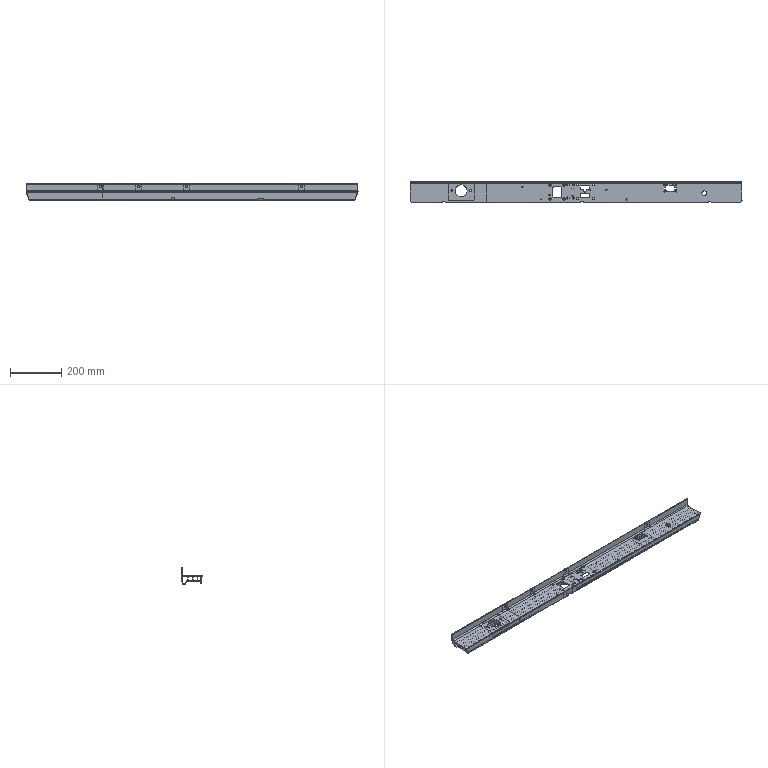NC program | NX | posted with a generic post | part box 1301 x 81.1 x 63 mm
Lines 16172 to 17479 of 19815:
(FIXED_CONTOUR , TOOL : R3)
N32324 T09 M6
N32326 G54
N32328 G17 G0 G90 X223.867 Y-31.775 B0. C0. S9500 M3
N32330 G43 Z30. H9
N32332 Z0.
N32334 G94 G1 Z-4.249 F1000.
N32336 G2 X223.567 Y-31.255 R0.6
N32338 G1 Y-31.038 Z-4.245 F2500.
N32340 Y-30.558
N32342 Y-30.373 Z-4.248
N32344 X223.574 Y-30.324 Z-4.256
N32346 X223.597 Y-30.217 Z-4.285
N32348 Y-30.558 Z-4.278
N32350 Y-31.039 Z-4.279
N32352 Y-31.409 Z-4.285
N32354 X223.635 Y-31.544 Z-4.331
N32356 Y-31.04 Z-4.321
N32358 Y-30.558 Z-4.32
N32360 Y-30.074 Z-4.33
N32362 Y-30.049 Z-4.332
N32364 X223.673 Y-29.89 Z-4.382
N32366 Y-30.074 Z-4.369
N32368 Y-30.412 Z-4.367
N32370 Y-30.558 Z-4.363
N32372 Y-31.041 Z-4.364
N32374 Y-31.187 Z-4.367
N32376 Y-31.526 Z-4.369
N32378 Y-31.675 Z-4.38
N32380 X223.685 Y-31.715 Z-4.394
N32382 X223.705 Y-31.774 Z-4.414
N32384 X223.743 Y-31.777 Z-4.448
N32386 Y-31.501 Z-4.44
N32388 Y-31.042 Z-4.434
N32390 Y-30.558
N32392 Y-30.049 Z-4.44
N32394 Y-29.82 Z-4.448
N32396 X223.815 Y-29.815 Z-4.51
N32398 Y-29.887 Z-4.507
N32400 Y-30.558 Z-4.504
N32402 Y-31.042
N32404 Y-31.766 Z-4.507
N32406 Y-31.783 Z-4.508
N32408 X223.873 Y-31.787 Z-4.556
N32410 X223.892 Y-31.788 Z-4.57
N32412 Y-31.224 Z-4.568
N32414 Y-29.912 Z-4.57
N32416 Y-29.811 Z-4.574
N32418 X223.901 Z-4.583
N32420 X223.971 Y-29.808 Z-4.629
N32422 Y-31.791 Z-4.63
N32424 X224.055 Y-31.795 Z-4.68
N32426 Y-30.074 Z-4.679
N32428 Y-29.804 Z-4.684
N32430 X224.093 Y-29.803 Z-4.707
N32432 X224.142 Y-29.802 Z-4.731
N32434 Y-30.015 Z-4.728
N32436 Y-31.797 Z-4.729
N32438 X224.231 Y-31.798 Z-4.774
N32440 Y-29.915 Z-4.773
N32442 Y-29.802 Z-4.775
N32444 X224.32 Y-29.801 Z-4.82
N32446 Y-31.799 Z-4.819
N32448 X224.339 Z-4.828
N32450 X224.412 Z-4.855
N32452 Y-29.888
N32454 Y-29.801 Z-4.858
N32456 X224.506 Y-29.8 Z-4.893
N32458 Y-29.992 Z-4.888
N32460 Y-31.8 Z-4.889
N32462 X224.583 Z-4.916
N32464 X224.601 Z-4.92
N32466 Y-30.049 Z-4.919
N32468 Y-29.8 Z-4.923
N32470 X224.698 Z-4.943
N32472 Y-29.939 Z-4.941
N32474 Y-31.8
N32476 X224.796 Z-4.963
N32478 Y-29.8
N32480 X224.895 Z-4.98
N32482 Y-29.882 Z-4.977
N32484 Y-31.718
N32486 Y-31.8 Z-4.979
N32488 X224.993 Z-4.995
N32490 Y-31.607 Z-4.988
N32492 Y-29.991
N32494 Y-29.8 Z-4.993
N32496 X225.067 Z-5.001
N32498 X225.093
N32500 Y-30.074 Z-4.998
N32502 Y-31.556 Z-4.997
N32504 Y-31.8 Z-5.001
N32506 X225.193
N32508 Y-31.669 Z-4.999
N32510 Y-31.537 Z-5.
N32512 Y-30.063
N32514 Y-29.931 Z-4.999
N32516 Y-29.8 Z-5.001
N32518 X225.293 Z-5.
N32520 Y-31.8
N32522 X225.393
N32524 Y-29.8
N32526 X225.493
N32528 Y-31.8
N32530 X225.593
N32532 Y-29.8
N32534 X225.693
N32536 Y-31.8
N32538 X225.793
N32540 Y-29.8
N32542 X225.893
N32544 Y-31.8
N32546 X225.993
N32548 Y-29.8
N32550 X226.093
N32552 Y-31.8
N32554 X226.193
N32556 Y-29.8
N32558 X226.293
N32560 Y-31.8
N32562 X226.393
N32564 Y-29.8
N32566 X226.493
N32568 Y-31.8
N32570 X226.593
N32572 Y-29.8
N32574 X226.693
N32576 Y-31.8
N32578 X226.793
N32580 Y-29.8
N32582 X226.893
N32584 Y-31.8
N32586 X226.993
N32588 Y-29.8
N32590 X227.093
N32592 Y-31.8
N32594 X227.193
N32596 Y-29.8
N32598 X227.293
N32600 Y-31.8
N32602 X227.393
N32604 Y-29.8
N32606 X227.493
N32608 Y-31.8
N32610 X227.593
N32612 Y-29.8
N32614 X227.693
N32616 Y-31.8
N32618 X227.793
N32620 Y-29.8
N32622 X227.893
N32624 Y-31.8
N32626 X227.993
N32628 Y-29.8
N32630 X228.093
N32632 Y-31.8
N32634 X228.193
N32636 Y-29.8
N32638 X228.293
N32640 Y-31.8
N32642 X228.393
N32644 Y-29.8
N32646 X228.493
N32648 Y-31.8
N32650 X228.593
N32652 Y-29.8
N32654 X228.693
N32656 Y-31.8
N32658 X228.793
N32660 Y-29.8
N32662 X228.893
N32664 Y-31.8
N32666 X228.993
N32668 Y-29.8
N32670 X229.093
N32672 Y-31.8
N32674 X229.193
N32676 Y-29.8
N32678 X229.293
N32680 Y-31.8
N32682 X229.393
N32684 Y-29.8
N32686 X229.493
N32688 Y-31.8
N32690 X229.593
N32692 Y-29.8
N32694 X229.693
N32696 Y-31.8
N32698 X229.793
N32700 Y-29.8
N32702 X229.893
N32704 Y-31.8
N32706 X229.993
N32708 Y-29.8
N32710 X230.093
N32712 Y-31.8
N32714 X230.193
N32716 Y-29.8
N32718 X230.293
N32720 Y-31.8
N32722 X230.393
N32724 Y-29.8
N32726 X230.493
N32728 Y-31.8
N32730 X230.593
N32732 Y-29.8
N32734 X230.693
N32736 Y-31.8
N32738 X230.793
N32740 Y-29.8
N32742 X230.893
N32744 Y-31.8
N32746 X230.993
N32748 Y-29.8
N32750 X231.093
N32752 Y-31.8
N32754 X231.193
N32756 Y-29.8
N32758 X231.293
N32760 Y-31.8
N32762 X231.393
N32764 Y-29.8
N32766 X231.493
N32768 Y-31.8
N32770 X231.593
N32772 Y-29.8
N32774 X231.693
N32776 Y-31.8
N32778 X231.793
N32780 Y-29.8
N32782 X231.893
N32784 Y-31.8
N32786 X231.993
N32788 Y-29.8
N32790 X232.093
N32792 Y-31.8
N32794 X232.193
N32796 Y-29.8
N32798 X232.293
N32800 Y-31.8
N32802 X232.393
N32804 Y-29.8
N32806 X232.493
N32808 Y-31.8
N32810 X232.593
N32812 Y-29.8
N32814 X232.693
N32816 Y-31.8
N32818 X232.793
N32820 Y-29.8
N32822 X232.893
N32824 Y-31.8
N32826 X232.993
N32828 Y-29.8
N32830 X233.093
N32832 Y-31.8
N32834 X233.193
N32836 Y-29.8
N32838 X233.293
N32840 Y-31.8
N32842 X233.393
N32844 Y-29.8
N32846 X233.493
N32848 Y-31.8
N32850 X233.593
N32852 Y-29.8
N32854 X233.693
N32856 Y-31.8
N32858 X233.793
N32860 Y-29.8
N32862 X233.893
N32864 Y-31.8
N32866 X233.993
N32868 Y-29.8
N32870 X234.093
N32872 Y-31.8
N32874 X234.193
N32876 Y-29.8
N32878 X234.293
N32880 Y-31.8
N32882 X234.393
N32884 Y-29.8
N32886 X234.493
N32888 Y-31.8
N32890 X234.593
N32892 Y-29.8
N32894 X234.693
N32896 Y-31.8
N32898 X234.793
N32900 Y-29.8
N32902 X234.893
N32904 Y-31.8
N32906 X234.993
N32908 Y-29.8
N32910 X235.093
N32912 Y-31.8
N32914 X235.193
N32916 Y-29.8
N32918 X235.293
N32920 Y-31.8
N32922 X235.393
N32924 Y-29.8
N32926 X235.493
N32928 Y-31.8
N32930 X235.593
N32932 Y-29.8
N32934 X235.693
N32936 Y-31.8
N32938 X235.793
N32940 Y-29.8
N32942 X235.893
N32944 Y-31.8
N32946 X235.993
N32948 Y-29.8
N32950 X236.093
N32952 Y-31.8
N32954 X236.193
N32956 Y-29.8
N32958 X236.293
N32960 Y-31.8
N32962 X236.393
N32964 Y-29.8
N32966 X236.493
N32968 Y-31.8
N32970 X236.593
N32972 Y-29.8
N32974 X236.693
N32976 Y-31.8
N32978 X236.793
N32980 Y-29.8
N32982 X236.893
N32984 Y-31.8
N32986 X236.993
N32988 Y-29.8
N32990 X237.093
N32992 Y-31.8
N32994 X237.193
N32996 Y-29.8
N32998 X237.293
N33000 Y-31.8
N33002 X237.393
N33004 Y-29.8
N33006 X237.493
N33008 Y-31.8
N33010 X237.593
N33012 Y-29.8
N33014 X237.693
N33016 Y-31.8
N33018 X237.793
N33020 Y-29.8
N33022 X237.893
N33024 Y-31.8
N33026 X237.993
N33028 Y-29.8
N33030 X238.093
N33032 Y-31.8
N33034 X238.193
N33036 Y-29.8
N33038 X238.293
N33040 Y-31.8
N33042 X238.393
N33044 Y-29.8
N33046 X238.493
N33048 Y-31.8
N33050 X238.593
N33052 Y-29.8
N33054 X238.693
N33056 Y-31.8
N33058 X238.793
N33060 Y-29.8
N33062 X238.893
N33064 Y-31.8
N33066 X238.993
N33068 Y-29.8
N33070 X239.093
N33072 Y-31.8
N33074 X239.193
N33076 Y-29.8
N33078 X239.293
N33080 Y-31.8
N33082 X239.393
N33084 Y-29.8
N33086 X239.493
N33088 Y-31.8
N33090 X239.593
N33092 Y-29.8
N33094 X239.693
N33096 Y-31.8
N33098 X239.793
N33100 Y-29.8
N33102 X239.893
N33104 Y-31.8
N33106 X239.993
N33108 Y-29.8
N33110 X240.093
N33112 Y-31.8
N33114 X240.193
N33116 Y-29.8
N33118 X240.293
N33120 Y-31.8
N33122 X240.393
N33124 Y-29.8
N33126 X240.493
N33128 Y-31.8
N33130 X240.593
N33132 Y-29.8
N33134 X240.693
N33136 Y-31.8
N33138 X240.793
N33140 Y-29.8
N33142 X240.893
N33144 Y-31.8
N33146 X240.993
N33148 Y-29.8
N33150 X241.093
N33152 Y-31.8
N33154 X241.193
N33156 Y-29.8
N33158 X241.293
N33160 Y-31.8
N33162 X241.393
N33164 Y-29.8
N33166 X241.493
N33168 Y-31.8
N33170 X241.593
N33172 Y-29.8
N33174 X241.693
N33176 Y-31.8
N33178 X241.793
N33180 Y-29.8
N33182 X241.893
N33184 Y-31.8
N33186 X241.993
N33188 Y-31.665 Z-4.999
N33190 Y-29.899
N33192 Y-29.8 Z-5.
N33194 X242.093 Z-5.001
N33196 Y-30.013 Z-4.998
N33198 Y-31.587
N33200 Y-31.8 Z-5.001
N33202 X242.148
N33204 X242.193 Z-4.996
N33206 Y-31.577 Z-4.992
N33208 Y-29.998
N33210 Y-29.8 Z-4.999
N33212 X242.291 Z-4.984
N33214 Y-29.912 Z-4.98
N33216 Y-31.688
N33218 Y-31.8 Z-4.984
N33220 X242.39 Z-4.969
N33222 Y-29.8
N33224 X242.488 Z-4.948
N33226 Y-31.691 Z-4.947
N33228 Y-31.8 Z-4.949
N33230 X242.586 Z-4.929
N33232 Y-31.581 Z-4.926
N33234 Y-29.8 Z-4.927
N33236 X242.638 Z-4.915
N33238 X242.682 Z-4.899
N33240 Y-31.578 Z-4.898
N33242 Y-31.8 Z-4.903
N33244 X242.775 Y-31.799 Z-4.869
N33246 Y-31.682 Z-4.865
N33248 Y-29.8
N33250 X242.868 Y-29.801 Z-4.832
N33252 Y-31.799
N33254 X242.957 Y-31.798 Z-4.789
N33256 Y-31.712 Z-4.787
N33258 Y-29.802 Z-4.788
N33260 X243.046 Y-29.803 Z-4.742
N33262 Y-31.612 Z-4.741
N33264 Y-31.797 Z-4.745
N33266 X243.135 Y-31.796 Z-4.699
N33268 Y-31.526 Z-4.695
N33270 Y-29.804 Z-4.696
N33272 X243.219 Y-29.808 Z-4.645
N33274 Y-31.526 Z-4.644
N33276 Y-31.793 Z-4.646
N33278 X243.3 Y-31.789 Z-4.592
N33280 Y-31.743
N33282 Y-31.643 Z-4.587
N33284 Y-29.957
N33286 Y-29.811 Z-4.588
N33288 X243.377 Y-29.815 Z-4.528
N33290 Y-31.042 Z-4.525
N33292 Y-31.785 Z-4.529
N33294 X243.449 Y-31.78 Z-4.468
N33296 Y-31.591 Z-4.46
N33298 Y-31.042 Z-4.456
N33300 Y-30.558
N33302 Y-29.991 Z-4.461
N33304 Y-29.821 Z-4.465
N33306 X243.521 Y-29.826 Z-4.404
N33308 Y-29.915 Z-4.402
N33310 Y-30.074 Z-4.39
N33312 Y-30.558 Z-4.387
N33314 Y-31.039
N33316 Y-31.526 Z-4.39
N33318 Y-31.685 Z-4.402
N33320 Y-31.774 Z-4.405
N33322 X243.524 Z-4.402
N33324 X243.535 Y-31.736 Z-4.391
N33326 X243.586 Y-31.527 Z-4.324
N33328 Y-30.948 Z-4.311
N33330 Y-30.558 Z-4.313
N33332 Y-30.073 Z-4.324
N33334 X243.641 Y-30.324 Z-4.256
N33336 X243.651 Y-30.403 Z-4.243
N33338 Y-30.637 Z-4.239
N33340 Y-30.854 Z-4.236
N33342 Y-31.197 Z-4.243
N33344 Y-27.737 Z-0.917
N33346 G0 Z30.
N33348 X571.432 Y-27.685
N33350 Z-1.2
N33352 G1 Z-2.475 F1000.
N33354 Y-31.294 Z-5.64
N33356 Y-31.017 Z-5.625 F2500.
N33358 Y-30.53 Z-5.626
N33360 Y-30.306 Z-5.638
N33362 X571.446 Y-30.155 Z-5.713
N33364 Y-30.53 Z-5.694
N33366 Y-31.017 Z-5.693
N33368 Y-31.451 Z-5.715
N33370 X571.451 Y-31.511 Z-5.743
N33372 X571.463 Y-31.565 Z-5.786
N33374 Y-31.503 Z-5.796
N33376 Y-31.354 Z-5.8
N33378 Y-31.017 Z-5.782
N33380 Y-30.53 Z-5.783
N33382 Y-30.131 Z-5.802
N33384 Y-30.044 Z-5.801
N33386 Y-30.015 Z-5.803
N33388 X571.471 Y-29.964 Z-5.844
N33390 X571.482 Y-29.926 Z-5.892
N33392 Y-29.972 Z-5.89
N33394 Y-30.044 Z-5.883
N33396 Y-30.348 Z-5.889
N33398 Y-30.53 Z-5.88
N33400 Y-31.017
N33402 Y-31.166 Z-5.888
N33404 Y-31.503 Z-5.881
N33406 Y-31.607 Z-5.866
N33408 Y-31.647 Z-5.857
N33410 X571.502 Y-31.714 Z-5.938
N33412 Y-31.668 Z-5.948
N33414 Y-31.503 Z-5.971
N33416 Y-31.136 Z-5.979
N33418 Y-30.53 Z-5.978
N33420 Y-30.449 Z-5.979
N33422 Y-30.044 Z-5.972
N33424 Y-30.007 Z-5.976
N33426 Y-29.954 Z-5.974
N33428 Y-29.875 Z-5.981
N33430 Y-29.864 Z-5.979
N33432 Y-29.854 Z-5.98
N33434 X571.515 Y-29.817 Z-6.028
N33436 X571.523 Y-29.815 Z-6.059
N33438 Y-29.864 Z-6.054
N33440 Y-29.925 Z-6.066
N33442 Y-29.954 Z-6.063
N33444 Y-30.049 Z-6.065
N33446 Y-30.53 Z-6.057
N33448 Y-31.017
N33450 Y-31.531 Z-6.062
N33452 Y-31.732 Z-6.034
N33454 Y-31.783 Z-6.023
N33456 X571.528 Y-31.799 Z-6.042
N33458 X571.545 Z-6.119
N33460 Y-31.648 Z-6.14
N33462 Y-31.503 Z-6.136
N33464 Y-31.273 Z-6.138
N33466 Y-31.017 Z-6.135
N33468 Y-30.53
N33470 Y-30.244 Z-6.14
N33472 Y-30.044 Z-6.139
N33474 Y-29.968 Z-6.144
N33476 Y-29.943
N33478 Y-29.864 Z-6.129
N33480 Y-29.81 Z-6.135
N33482 X571.567 Y-29.805 Z-6.214
N33484 Y-29.864 Z-6.207
N33486 Y-29.918 Z-6.217
N33488 Y-30.003 Z-6.218
N33490 Y-30.044 Z-6.215
N33492 Y-30.454 Z-6.218
N33494 Y-31.017 Z-6.217
N33496 Y-31.503 Z-6.214
N33498 Y-31.769 Z-6.222
N33500 Y-31.8 Z-6.218
N33502 X571.593 Z-6.315
N33504 Y-31.62 Z-6.31
N33506 Y-31.503 Z-6.303
N33508 Y-31.468 Z-6.304
N33510 Y-30.53 Z-6.302
N33512 Y-29.954 Z-6.304
N33514 Y-29.887 Z-6.303
N33516 Y-29.864 Z-6.299
N33518 Y-29.8 Z-6.306
N33520 X571.612 Y-29.801 Z-6.373
N33522 X571.623 Z-6.402
N33524 Y-29.938 Z-6.39
N33526 Y-30.044 Z-6.387
N33528 Y-30.293 Z-6.395
N33530 Y-31.239
N33532 Y-31.503 Z-6.385
N33534 Y-31.575
N33536 Y-31.8 Z-6.4
N33538 X571.654 Z-6.482
N33540 Y-31.641 Z-6.472
N33542 Y-31.503
N33544 Y-31.031 Z-6.489
N33546 Y-30.517
N33548 Y-30.044 Z-6.473
N33550 Y-29.991 Z-6.475
N33552 Y-29.916
N33554 Y-29.864 Z-6.479
N33556 Y-29.8 Z-6.481
N33558 X571.688 Z-6.571
N33560 Y-29.892 Z-6.567
N33562 Y-30.044 Z-6.566
N33564 Y-30.303 Z-6.575
N33566 Y-31.245
N33568 Y-31.503 Z-6.566
N33570 Y-31.713
N33572 Y-31.8 Z-6.571
N33574 X571.722 Z-6.661
N33576 Y-31.503 Z-6.66
N33578 Y-31.459 Z-6.661
N33580 Y-30.088
N33582 Y-29.869 Z-6.66
N33584 Y-29.8 Z-6.661
N33586 X571.759 Z-6.753
N33588 Y-31.728 Z-6.752
N33590 Y-31.8 Z-6.754
N33592 X571.795 Z-6.847
N33594 Y-31.639 Z-6.843
N33596 Y-29.932
N33598 Y-29.8 Z-6.845
N33600 X571.832 Z-6.937
N33602 Y-30.005 Z-6.933
N33604 Y-31.55
N33606 Y-31.8 Z-6.94
N33608 X571.851 Z-6.99
N33610 X571.872 Z-7.031
N33612 Y-31.503 Z-7.023
N33614 Y-30.044
N33616 Y-29.8 Z-7.028
N33618 X571.918 Z-7.117
N33620 Y-30.044 Z-7.112
N33622 Y-31.503
N33624 Y-31.8 Z-7.12
N33626 X571.963 Z-7.209
N33628 Y-31.503 Z-7.201
N33630 Y-30.044
N33632 Y-29.8 Z-7.206
N33634 X572.009 Z-7.295
N33636 Y-30.044 Z-7.29
N33638 Y-31.503
N33640 Y-31.8 Z-7.298
N33642 X572.056 Z-7.386
N33644 Y-31.503 Z-7.378
N33646 Y-30.044
N33648 Y-29.8 Z-7.383
N33650 X572.103 Z-7.471
N33652 Y-30.027 Z-7.466
N33654 Y-31.523
N33656 Y-31.8 Z-7.473
N33658 X572.157 Z-7.554
N33660 Y-31.654 Z-7.551
N33662 Y-29.919
N33664 Y-29.8 Z-7.554
N33666 X572.211 Z-7.635
N33668 Y-31.8
N33670 X572.265 Z-7.719
N33672 Y-31.741 Z-7.715
N33674 Y-29.849
N33676 Y-29.8 Z-7.717
N33678 X572.32 Z-7.798
N33680 Y-29.903 Z-7.795
N33682 Y-31.674
N33684 Y-31.8 Z-7.802
N33686 X572.375 Z-7.881
N33688 Y-31.673 Z-7.879
N33690 Y-31.607 Z-7.875
N33692 Y-29.958
N33694 Y-29.8 Z-7.878
N33696 X572.431 Z-7.959
N33698 Y-30.014 Z-7.956
N33700 Y-31.539
N33702 Y-31.8 Z-7.962
N33704 X572.461 Z-8.005
N33706 X572.49 Z-8.042
N33708 Y-31.539 Z-8.036
N33710 Y-30. Z-8.037
N33712 Y-29.8 Z-8.039
N33714 X572.552 Z-8.117
N33716 Y-29.952 Z-8.115
N33718 Y-31.615
N33720 Y-31.8 Z-8.118
N33722 X572.615 Z-8.195
N33724 Y-31.69 Z-8.193
N33726 Y-29.889
N33728 Y-29.8 Z-8.195
N33730 X572.677 Z-8.272
N33732 Y-31.8
N33734 X572.705 Z-8.307
N33736 X572.742 Z-8.348
N33738 Y-31.755 Z-8.346
N33740 Y-29.8 Z-8.347
N33742 X572.809 Z-8.42
N33744 Y-29.904 Z-8.417
N33746 Y-31.673
N33748 Y-31.8 Z-8.422
N33750 X572.876 Z-8.493
N33752 Y-31.591 Z-8.488
N33754 Y-29.971
N33756 Y-29.8 Z-8.493
N33758 X572.944 Z-8.566
N33760 Y-30.037 Z-8.559
N33762 Y-31.512
N33764 Y-31.8 Z-8.565
N33766 X573.015 Z-8.631
N33768 Y-31.584 Z-8.627
N33770 Y-29.977 Z-8.63
N33772 Y-29.797 Z-8.635
N33774 X573.086 Y-29.794 Z-8.704
N33776 Y-29.906 Z-8.701
N33778 Y-31.67 Z-8.694
N33780 Y-31.8 Z-8.696
N33782 X573.157 Z-8.762
N33784 Y-29.79 Z-8.773
N33786 X573.192 Y-29.789 Z-8.807
N33788 X573.231 Y-29.78 Z-8.84
N33790 Y-31.8 Z-8.829
N33792 X573.305 Z-8.895
N33794 Y-31.663 Z-8.893
N33796 Y-29.912 Z-8.901
N33798 Y-29.763 Z-8.904
N33800 X573.38 Y-29.746 Z-8.968
N33802 Y-30.044 Z-8.962
N33804 Y-31.572 Z-8.959
N33806 Y-31.8 Z-8.962
N33808 X573.436 Z-9.012
N33810 X573.456 Z-9.027
N33812 Y-31.527 Z-9.022
N33814 Y-30.014 Z-9.025
N33816 Y-29.729 Z-9.031
N33818 X573.536 Y-29.712 Z-9.089
N33820 Y-29.895 Z-9.085
N33822 Y-30.331 Z-9.084
N33824 Y-30.53 Z-9.082
N33826 Y-31.625 Z-9.08
N33828 Y-31.8 Z-9.084
N33830 X573.616 Z-9.14
N33832 Y-31.722 Z-9.137
N33834 Y-30.53 Z-9.14
N33836 Y-30.044 Z-9.144
N33838 Y-29.784 Z-9.145
N33840 Y-29.695 Z-9.147
N33842 X573.68 Y-29.681 Z-9.193
N33844 X573.697 Y-29.675 Z-9.204
N33846 Y-30.078 Z-9.203
N33848 Y-30.564 Z-9.197
N33850 Y-31.779 Z-9.194
N33852 Y-31.8 Z-9.195
N33854 X573.779 Z-9.252
N33856 Y-31.68 Z-9.25
N33858 Y-30.53 Z-9.252
N33860 Y-30.241 Z-9.256
N33862 Y-29.645 Z-9.258
N33864 X573.861 Y-29.615 Z-9.312
N33866 Y-30.53 Z-9.307
N33868 Y-31.58 Z-9.306
N33870 Y-31.8 Z-9.31
N33872 X573.924 Z-9.354
N33874 X573.944 Z-9.365
N33876 Y-31.527 Z-9.361
N33878 Y-30.044 Z-9.362
N33880 Y-29.572 Z-9.367
N33882 X573.991 Y-29.545 Z-9.397
N33884 X574.028 Y-29.524 Z-9.419
N33886 Y-30.251 Z-9.412
N33888 Y-31.63 Z-9.41
N33890 Y-31.8 Z-9.414
N33892 X574.113 Z-9.462
N33894 Y-31.733 Z-9.459
N33896 Y-30.907
N33898 Y-29.557 Z-9.469
N33900 Y-29.477
N33902 X574.168 Y-29.446 Z-9.501
N33904 X574.2 Y-29.425 Z-9.518
N33906 Y-31.017 Z-9.508
N33908 Y-31.8 Z-9.509
N33910 X574.287 Z-9.557
N33912 Y-31.655 Z-9.555
N33914 Y-30.53 Z-9.557
N33916 Y-29.506 Z-9.562
N33918 Y-29.368 Z-9.566
N33920 X574.373 Y-29.311 Z-9.612
N33922 Y-29.54 Z-9.606
N33924 Y-30.044 Z-9.602
N33926 Y-31.55 Z-9.601
N33928 Y-31.8 Z-9.605
N33930 X574.412 Z-9.626
N33932 X574.46 Z-9.648
N33934 Y-31.562 Z-9.644
N33936 Y-29.948 Z-9.646
N33938 Y-29.461 Z-9.649
N33940 Y-29.255 Z-9.654
N33942 X574.549 Y-29.198 Z-9.694
N33944 Y-29.317 Z-9.691
N33946 Y-30.803 Z-9.684
N33948 Y-31.67
N33950 Y-31.8 Z-9.688
N33952 X574.638 Z-9.726
N33954 Y-30.982
N33956 Y-29.557 Z-9.734
N33958 Y-29.141 Z-9.735
N33960 X574.655 Y-29.13 Z-9.742
N33962 X574.729 Y-29.065 Z-9.774
N33964 X574.73 Y-30.044 Z-9.769
N33966 Y-31.017 Z-9.764
N33968 Y-31.8 Z-9.765
N33970 X574.821 Z-9.805
N33972 Y-31.598 Z-9.802
N33974 Y-29.557 Z-9.806
N33976 Y-28.986 Z-9.808
N33978 X574.913 Y-28.906 Z-9.842
N33980 Y-30.071 Z-9.839
N33982 Y-31.53 Z-9.84
N33984 Y-31.8 Z-9.843
N33986 X575.006 Z-9.875
N33988 Y-31.632 Z-9.871
N33990 Y-30.256 Z-9.872
N33992 Y-29.071 Z-9.876
N33994 Y-28.827 Z-9.877
N33996 X575.098 Y-28.747 Z-9.911
N33998 Y-30.044 Z-9.908
N34000 Y-30.53 Z-9.904
N34002 Y-31.745 Z-9.903
N34004 Y-31.8 Z-9.905
N34006 X575.192 Z-9.935
N34008 Y-30.53
N34010 Y-29.654 Z-9.94
N34012 Y-28.661 Z-9.943
N34014 X575.284 Y-28.551 Z-9.972
N34016 Y-29.352 Z-9.966
N34018 Y-30.324 Z-9.965
N34020 Y-31.017 Z-9.963
N34022 Y-31.629
N34024 Y-31.8 Z-9.965
N34026 X575.376 Z-9.995
N34028 Y-31.517 Z-9.991
N34030 Y-29.535
N34032 Y-28.585 Z-9.995
N34034 Y-28.441 Z-9.999
N34036 X575.391 Y-28.423 Z-10.004
N34038 X575.462 Y-28.315 Z-10.025
N34040 Y-28.585 Z-10.018
N34042 Y-30.193 Z-10.013
N34044 Y-31.594
N34046 Y-31.8 Z-10.016
N34048 X575.548 Z-10.037
N34050 Y-31.698 Z-10.033
N34052 Y-29.877 Z-10.035
N34054 Y-28.585 Z-10.04
N34056 Y-28.428 Z-10.045
N34058 Y-28.187
N34060 X575.554 Y-28.178 Z-10.046
N34062 X575.622 Y-28.033 Z-10.061
N34064 Y-29.54 Z-10.057
N34066 Y-30.512 Z-10.052
N34068 Y-31.8
N34070 X575.719 Z-10.076
N34072 Y-31.693 Z-10.073
N34074 Y-30.044 Z-10.074
N34076 Y-29.071 Z-10.078
N34078 Y-27.978 Z-10.08
N34080 X575.816 Y-27.937 Z-10.097
N34082 Y-28.078 Z-10.096
N34084 Y-31.574 Z-10.094
N34086 Y-31.8 Z-10.099
N34088 X575.875 Z-10.11
N34090 X575.915 Z-10.115
N34092 Y-31.551 Z-10.112
N34094 Y-27.896
N34096 X576.013 Y-27.854 Z-10.126
N34098 Y-31.671
N34100 Y-31.8 Z-10.128
N34102 X576.112 Z-10.141
N34104 Y-27.813 Z-10.14
N34106 X576.119 Y-27.81 Z-10.142
N34108 X576.21 Y-27.807 Z-10.158
N34110 Y-27.911 Z-10.155
N34112 Y-31.689
N34114 Y-31.8 Z-10.158
N34116 X576.309 Z-10.172
N34118 Y-31.569 Z-10.169
N34120 Y-28.032
N34122 Y-27.804 Z-10.172
N34124 X576.363 Y-27.803 Z-10.18
N34126 X576.408 Y-27.802 Z-10.183
N34128 Y-28.043 Z-10.18
N34130 Y-31.558
N34132 Y-31.8 Z-10.183
N34134 X576.508 Z-10.188
N34136 Y-31.68 Z-10.187
N34138 Y-27.921
N34140 Y-27.802 Z-10.188
N34142 X576.606 Y-27.801 Z-10.193
N34144 X576.608 Y-31.8
N34146 X576.707 Z-10.197
N34148 Y-31.677 Z-10.196
N34150 Y-27.923
N34152 Y-27.802 Z-10.197
N34154 X576.807 Z-10.201
N34156 Y-28.046 Z-10.198
N34158 Y-31.555
N34160 Y-31.8 Z-10.201
N34162 X576.851 Z-10.203
N34164 X576.907 Z-10.2
N34166 Y-31.572 Z-10.198
N34168 Y-28.029
N34170 Y-27.802 Z-10.2
N34172 X577.007 Z-10.197
N34174 Y-31.694 Z-10.195
N34176 Y-31.8 Z-10.197
N34178 X577.107 Z-10.193
N34180 Y-27.803
N34182 X577.207 Y-27.804 Z-10.189
N34184 Y-27.938 Z-10.186
N34186 Y-31.663
N34188 Y-31.8 Z-10.189
N34190 X577.307 Z-10.182
N34192 Y-31.541 Z-10.179
N34194 Y-28.036 Z-10.18
N34196 Y-27.806 Z-10.182
N34198 X577.338 Z-10.18
N34200 X577.406 Y-27.807 Z-10.169
N34202 Y-28.016 Z-10.167
N34204 Y-31.585
N34206 Y-31.8 Z-10.17
N34208 X577.505 Z-10.154
N34210 Y-27.809
N34212 X577.582 Y-27.81 Z-10.142
N34214 X577.604 Y-27.819 Z-10.139
N34216 Y-31.8
N34218 X577.703 Z-10.126
N34220 Y-31.654 Z-10.124
N34222 Y-27.86
N34224 X577.801 Y-27.901 Z-10.109
N34226 Y-31.533 Z-10.11
N34228 Y-31.8 Z-10.113
N34230 X577.826 Z-10.11
N34232 X577.899 Z-10.093
N34234 Y-31.592 Z-10.09
N34236 Y-28.072 Z-10.093
N34238 Y-27.941 Z-10.095
N34240 X577.997 Y-27.982 Z-10.077
N34242 Y-29.703 Z-10.074
N34244 Y-30.53 Z-10.069
N34246 Y-31.8 Z-10.071
N34248 X578.094 Z-10.048
N34250 Y-30.482
N34252 Y-29.071 Z-10.055
N34254 Y-28.065 Z-10.057
N34256 X578.147 Y-28.178 Z-10.044
N34258 X578.191 Y-28.244 Z-10.032
N34260 Y-30.289 Z-10.024
N34262 Y-31.653
N34264 Y-31.8 Z-10.026
N34266 X578.287 Z-10.004
N34268 Y-31.535 Z-10.001
N34270 Y-29.557
N34272 Y-28.39 Z-10.006
N34274 X578.309 Y-28.423 Z-10.
N34276 X578.383 Y-28.511 Z-9.98
N34278 Y-29.696 Z-9.974
N34280 Y-31.587 Z-9.973
N34282 Y-31.8 Z-9.976
N34284 X578.478 Z-9.945
N34286 Y-30.53 Z-9.944
N34288 Y-30.202 Z-9.947
N34290 Y-29.071 Z-9.95
N34292 Y-28.626 Z-9.953
N34294 X578.511 Y-28.662 Z-9.943
N34296 X578.574 Y-28.722 Z-9.922
N34298 Y-30.044 Z-9.918
N34300 Y-30.499 Z-9.914
N34302 Y-31.8
N34304 X578.667 Z-9.883
N34306 Y-31.667 Z-9.881
N34308 Y-30.312
N34310 Y-29.071 Z-9.887
N34312 Y-28.803
N34314 X578.761 Y-28.884 Z-9.852
N34316 Y-30.125 Z-9.848
N34318 Y-31.552
N34320 Y-31.8 Z-9.852
N34322 X578.802 Z-9.838
N34324 X578.854 Z-9.815
N34326 Y-31.567 Z-9.812
N34328 Y-29.557 Z-9.815
N34330 Y-28.964 Z-9.818
N34332 X578.946 Y-29.043 Z-9.784
N34334 Y-30.044 Z-9.779
N34336 Y-31.017 Z-9.775
N34338 Y-31.679
N34340 Y-31.8 Z-9.776
N34342 X579.038 Z-9.737
N34344 Y-31.017
N34346 Y-30.058 Z-9.743
N34348 Y-29.123 Z-9.746
N34350 X579.045 Y-29.13 Z-9.743
N34352 X579.128 Y-29.183 Z-9.705
N34354 Y-29.879 Z-9.702
N34356 Y-30.53 Z-9.697
N34358 Y-30.851 Z-9.696
N34360 Y-31.699
N34362 Y-31.8 Z-9.699
N34364 X579.218 Z-9.658
N34366 Y-31.59 Z-9.654
N34368 Y-30.186 Z-9.655
N34370 Y-29.415 Z-9.66
N34372 Y-29.24 Z-9.664
N34374 X579.308 Y-29.298 Z-9.622
N34376 Y-29.594 Z-9.616
N34378 Y-30.044 Z-9.612
N34380 Y-31.525
N34382 Y-31.8 Z-9.615
N34384 X579.395 Z-9.567
N34386 Y-31.632 Z-9.565
N34388 Y-30.53 Z-9.566
N34390 Y-29.514 Z-9.572
N34392 Y-29.356 Z-9.576
N34394 X579.483 Y-29.413 Z-9.528
N34396 Y-29.557 Z-9.527
N34398 Y-31.017 Z-9.518
N34400 Y-31.8 Z-9.519
N34402 X579.57 Z-9.471
N34404 Y-31.755 Z-9.47
N34406 Y-30.943
N34408 Y-29.557 Z-9.479
N34410 Y-29.467
N34412 X579.656 Y-29.515 Z-9.429
N34414 Y-30.286 Z-9.422
N34416 Y-30.773 Z-9.42
N34418 Y-31.651
N34420 Y-31.8 Z-9.424
N34422 X579.741 Z-9.374
N34424 Y-31.547 Z-9.37
N34426 Y-30.044 Z-9.372
N34428 Y-29.563 Z-9.377
N34430 X579.824 Y-29.61 Z-9.322
N34432 Y-30.53 Z-9.317
N34434 Y-31.561
N34436 Y-31.8 Z-9.32
N34438 X579.906 Z-9.263
N34440 Y-31.503 Z-9.261
N34442 Y-30.53 Z-9.263
N34444 Y-30.272 Z-9.266
N34446 Y-29.646 Z-9.268
N34448 X579.988 Y-29.673 Z-9.214
N34450 Y-30.109 Z-9.213
N34452 Y-30.595 Z-9.208
N34454 Y-31.76 Z-9.205
N34456 Y-31.8
N34458 X580.07 Z-9.15
N34460 Y-31.741 Z-9.148
N34462 Y-30.53 Z-9.151
N34464 Y-30.141 Z-9.155
N34466 Y-29.762 Z-9.156
N34468 Y-29.694 Z-9.158
N34470 X580.15 Y-29.711 Z-9.1
N34472 Y-29.874 Z-9.096
N34474 Y-30.301 Z-9.095
N34476 Y-30.759 Z-9.091
N34478 Y-31.643 Z-9.09
N34480 Y-31.8 Z-9.095
N34482 X580.23 Z-9.037
N34484 Y-31.545 Z-9.033
N34486 Y-29.992 Z-9.036
N34488 Y-29.728 Z-9.042
N34490 X580.265 Y-29.735 Z-9.016
N34492 X580.308 Y-29.744 Z-8.98
N34494 Y-30.044 Z-8.974
N34496 Y-31.555 Z-8.97
N34498 Y-31.8 Z-8.974
N34500 X580.382 Z-8.907
N34502 Y-31.646 Z-8.905
N34504 Y-29.926 Z-8.912
N34506 Y-29.761 Z-8.915
N34508 X580.457 Y-29.777 Z-8.851
N34510 Y-31.8 Z-8.841
N34512 X580.531 Z-8.774
N34514 Y-29.79 Z-8.785
N34516 X580.602 Y-29.793 Z-8.717
N34518 Y-29.893 Z-8.714
N34520 Y-31.686 Z-8.706
N34522 Y-31.8 Z-8.708
N34524 X580.673 Z-8.643
N34526 Y-31.6 Z-8.639
N34528 Y-29.964 Z-8.643
N34530 Y-29.796 Z-8.648
N34532 X580.744 Y-29.799 Z-8.58
N34534 Y-30.044 Z-8.573
N34536 Y-31.513 Z-8.572
N34538 Y-31.8 Z-8.577
N34540 X580.813 Z-8.506
N34542 Y-31.576 Z-8.501
N34544 Y-29.984
N34546 Y-29.8 Z-8.506
N34548 X580.88 Z-8.433
N34550 Y-29.917 Z-8.43
N34552 Y-31.658
N34554 Y-31.8 Z-8.435
N34556 X580.947 Z-8.362
N34558 Y-31.739 Z-8.359
N34560 Y-29.85
N34562 Y-29.8 Z-8.36
N34564 X580.997 Z-8.306
N34566 X581.012 Z-8.286
N34568 Y-31.8
N34570 X581.075 Z-8.21
N34572 Y-31.705 Z-8.208
N34574 Y-29.8 Z-8.209
N34576 X581.137 Z-8.131
N34578 Y-30.044 Z-8.129
N34580 Y-31.629
N34582 Y-31.8 Z-8.133
N34584 X581.199 Z-8.056
N34586 Y-31.553 Z-8.051
N34588 Y-30.044
N34590 Y-29.8 Z-8.053
N34592 X581.242 Z-7.999
N34594 X581.259 Z-7.974
N34596 Y-30.025 Z-7.971
N34598 Y-31.54 Z-7.972
N34600 Y-31.8 Z-7.977
N34602 X581.315 Z-7.897
N34604 Y-31.652 Z-7.894
N34606 Y-31.594 Z-7.89
N34608 Y-29.969
N34610 Y-29.8 Z-7.893
N34612 X581.37 Z-7.813
N34614 Y-29.914 Z-7.81
N34616 Y-31.661
N34618 Y-31.8 Z-7.817
N34620 X581.425 Z-7.735
N34622 Y-31.728 Z-7.731
N34624 Y-29.859
N34626 Y-29.8 Z-7.733
N34628 X581.48 Z-7.651
N34630 Y-31.8
N34632 X581.534 Z-7.569
N34634 Y-31.679 Z-7.567
N34636 Y-29.899
N34638 Y-29.8 Z-7.57
N34640 X581.587 Z-7.485
N34642 Y-30.006 Z-7.482
N34644 Y-31.549
N34646 Y-31.8 Z-7.488
N34648 X581.606 Z-7.459
N34650 X581.636 Z-7.402
N34652 Y-31.503 Z-7.395
N34654 Y-30.044
N34656 Y-29.8 Z-7.398
N34658 X581.683 Z-7.31
N34660 Y-30.044 Z-7.307
N34662 Y-31.503
N34664 Y-31.8 Z-7.315
N34666 X581.729 Z-7.226
N34668 Y-31.503 Z-7.218
N34670 Y-30.04
N34672 Y-29.8 Z-7.222
N34674 X581.775 Z-7.133
N34676 Y-30.044 Z-7.129
N34678 Y-31.503
N34680 Y-31.8 Z-7.137
N34682 X581.82 Z-7.048
N34684 Y-31.503 Z-7.04
N34686 Y-30.044
N34688 Y-29.8 Z-7.044
N34690 X581.85 Z-6.984
N34692 X581.862 Z-6.953
N34694 Y-30.019 Z-6.95
N34696 Y-31.533
N34698 Y-31.8 Z-6.957
N34700 X581.899 Z-6.864
N34702 Y-31.622 Z-6.859
N34704 Y-29.946
N34706 Y-29.8 Z-6.862
N34708 X581.936 Z-6.77
N34710 Y-31.711 Z-6.769
N34712 Y-31.8 Z-6.771
N34714 X581.972 Z-6.679
N34716 Y-29.8 Z-6.678
N34718 X582.006 Z-6.591
N34720 Y-29.84 Z-6.587
N34722 Y-30.41 Z-6.586
N34724 Y-30.53 Z-6.584
N34726 Y-31.017
N34728 Y-31.133 Z-6.585
N34730 Y-31.729
N34732 Y-31.8 Z-6.59
N34734 X582.039 Z-6.502
N34736 Y-31.658 Z-6.493
N34738 Y-31.25
N34740 Y-31.017 Z-6.49
N34742 Y-30.53
N34744 Y-30.291 Z-6.493
N34746 Y-30.044
N34748 Y-29.997 Z-6.495
N34750 Y-29.88
N34752 Y-29.8 Z-6.503
N34754 X582.073 Z-6.416
N34756 Y-29.921 Z-6.404
N34758 Y-29.973
N34760 Y-30.044 Z-6.401
N34762 Y-30.171
N34764 Y-30.53 Z-6.396
N34766 Y-31.017 Z-6.395
N34768 Y-31.366 Z-6.4
N34770 Y-31.587
N34772 Y-31.8 Z-6.414
N34774 X582.101 Z-6.34
N34776 X582.106 Z-6.322
N34778 Y-31.664 Z-6.318
N34780 Y-31.516 Z-6.308
N34782 Y-31.017 Z-6.302
N34784 Y-30.53
N34786 Y-30.017 Z-6.31
N34788 Y-29.954
N34790 Y-29.8 Z-6.323
N34792 X582.135 Z-6.229
N34794 Y-29.954 Z-6.216
N34796 Y-30.003
N34798 Y-30.044 Z-6.213
N34800 Y-30.449 Z-6.217
N34802 Y-30.53 Z-6.215
N34804 Y-31.086 Z-6.216
N34806 Y-31.503 Z-6.213
N34808 Y-31.767 Z-6.221
N34810 Y-31.8 Z-6.216
N34812 X582.157 Y-31.799 Z-6.118
N34814 Y-31.646 Z-6.139
N34816 Y-31.503 Z-6.134
N34818 Y-31.277 Z-6.136
N34820 Y-31.017 Z-6.133
N34822 Y-30.53
N34824 Y-30.239 Z-6.139
N34826 Y-30.044 Z-6.137
N34828 Y-29.907 Z-6.146
N34830 Y-29.8 Z-6.139
N34832 X582.178 Y-29.801 Z-6.051
N34834 Y-29.803 Z-6.049
N34836 Y-29.954 Z-6.059
N34838 Y-30.066 Z-6.061
N34840 Y-30.53 Z-6.053
N34842 Y-31.017
N34844 Y-31.527 Z-6.058
N34846 Y-31.731 Z-6.031
N34848 Y-31.76 Z-6.025
N34850 X582.19 Y-31.739 Z-5.977
N34852 X582.2 Y-31.707 Z-5.935
N34854 Y-31.666 Z-5.944
N34856 Y-31.503 Z-5.966
N34858 Y-31.112 Z-5.974
N34860 Y-30.466
N34862 Y-30.044 Z-5.968
N34864 Y-30.005 Z-5.971
N34866 Y-29.954 Z-5.97
N34868 Y-29.868 Z-5.964
N34870 X582.22 Y-29.932 Z-5.885
N34872 Y-29.971 Z-5.887
N34874 Y-30.044 Z-5.88
N34876 Y-30.34 Z-5.885
N34878 Y-30.53 Z-5.875
N34880 Y-31.017 Z-5.876
N34882 Y-31.173 Z-5.884
N34884 Y-31.503 Z-5.877
N34886 Y-31.605 Z-5.863
N34888 Y-31.643 Z-5.855
N34890 X582.224 Y-31.63 Z-5.838
N34892 X582.239 Y-31.561 Z-5.783
N34894 Y-31.503 Z-5.792
N34896 Y-31.361 Z-5.795
N34898 Y-31.017 Z-5.777
N34900 Y-30.53 Z-5.778
N34902 Y-30.122 Z-5.798
N34904 Y-30.044 Z-5.797
N34906 Y-30.02 Z-5.799
N34908 X582.249 Y-30.082 Z-5.748
N34910 X582.258 Y-30.184 Z-5.698
N34912 Y-30.53 Z-5.68
N34914 Y-31.017 Z-5.679
N34916 Y-31.421 Z-5.7
N34918 X582.27 Y-31.273 Z-5.629
N34920 X582.277 Y-31.097 Z-5.585
N34922 Y-31.017 Z-5.581
N34924 Y-30.505 Z-5.584
N34926 G3 X581.977 Y-29.985 R0.6
N34928 G1 Z0.
N34930 G0 Z30.
N34932 M5